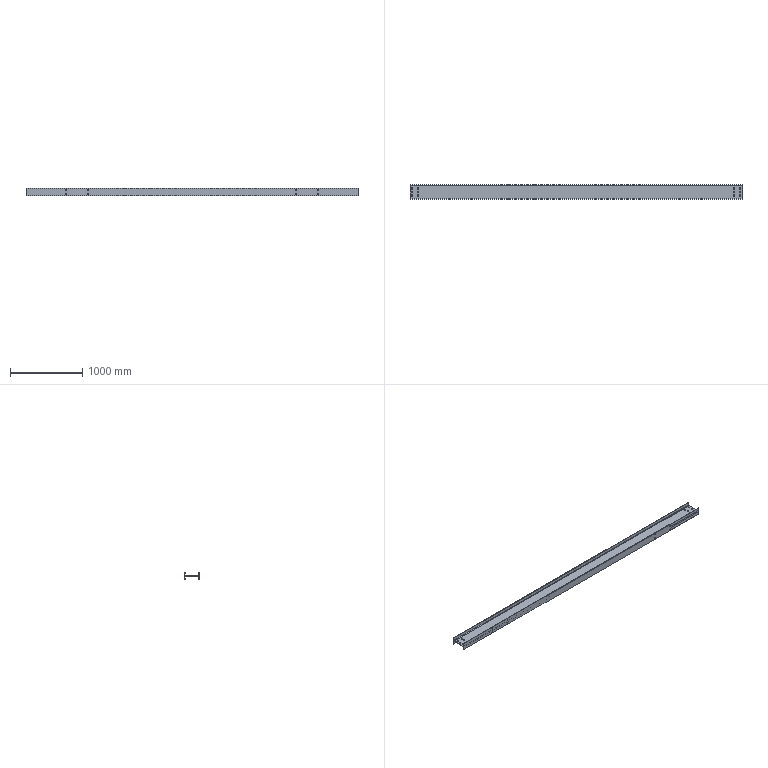Part | STEP file | 休息台主梁3主体_Default<As Machined> | 1 solid | 58 faces | box 4586 x 200 x 100 mm | volume 12200555 mm3 | cylinder 44 | plane 14 | commonest cylinder face diameters 19 x24 15 x16 16 x4